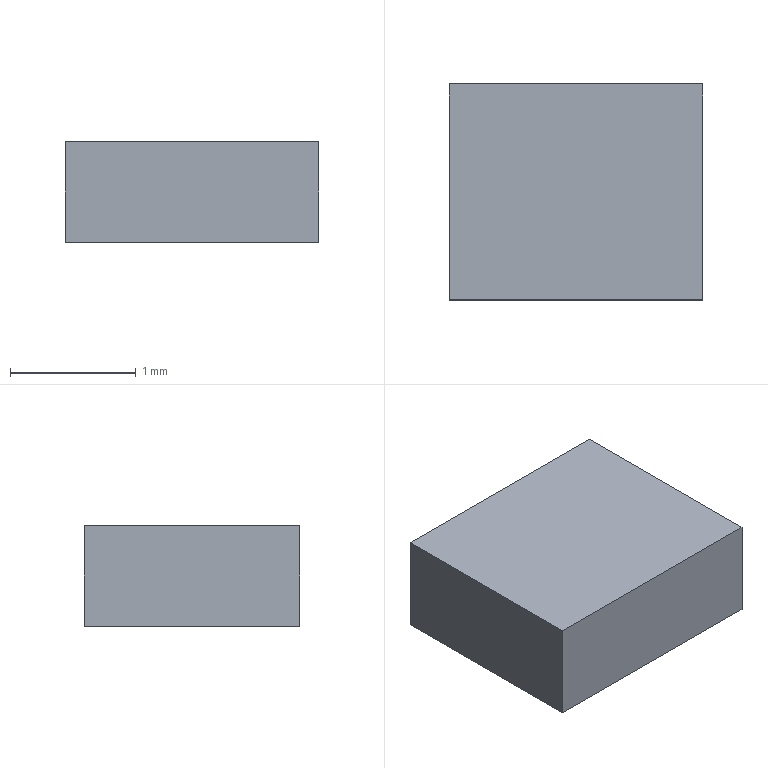Part | Creo | 1 solid | 6 faces | box 2.02 x 1.72 x 0.8 mm | volume 2.78 mm3 | plane 6
STEP:
#1=CARTESIAN_POINT('',(0.,0.,0.));
#2=DIRECTION('',(0.,0.,1.));
#3=DIRECTION('',(1.,0.,0.));
#4=AXIS2_PLACEMENT_3D('',#1,#2,#3);
#5=CARTESIAN_POINT('',(-1.01,-0.86,0.));
#6=VERTEX_POINT('',#5);
#7=CARTESIAN_POINT('',(1.01,-0.86,0.));
#8=VERTEX_POINT('',#7);
#9=CARTESIAN_POINT('',(-1.01,-0.86,0.));
#10=DIRECTION('',(1.,0.,0.));
#11=VECTOR('',#10,2.02);
#12=LINE('',#9,#11);
#13=EDGE_CURVE('',#6,#8,#12,.T.);
#14=ORIENTED_EDGE('',*,*,#13,.T.);
#15=CARTESIAN_POINT('',(1.01,0.86,0.));
#16=VERTEX_POINT('',#15);
#17=CARTESIAN_POINT('',(1.01,-0.86,0.));
#18=DIRECTION('',(0.,1.,0.));
#19=VECTOR('',#18,1.72);
#20=LINE('',#17,#19);
#21=EDGE_CURVE('',#8,#16,#20,.T.);
#22=ORIENTED_EDGE('',*,*,#21,.T.);
#23=CARTESIAN_POINT('',(-1.01,0.86,0.));
#24=VERTEX_POINT('',#23);
#25=CARTESIAN_POINT('',(1.01,0.86,0.));
#26=DIRECTION('',(-1.,0.,0.));
#27=VECTOR('',#26,2.02);
#28=LINE('',#25,#27);
#29=EDGE_CURVE('',#16,#24,#28,.T.);
#30=ORIENTED_EDGE('',*,*,#29,.T.);
#31=CARTESIAN_POINT('',(-1.01,0.86,0.));
#32=DIRECTION('',(0.,-1.,0.));
#33=VECTOR('',#32,1.72);
#34=LINE('',#31,#33);
#35=EDGE_CURVE('',#24,#6,#34,.T.);
#36=ORIENTED_EDGE('',*,*,#35,.T.);
#37=EDGE_LOOP('',(#14,#22,#30,#36));
#38=FACE_OUTER_BOUND('',#37,.F.);
#39=CARTESIAN_POINT('',(0.,0.,0.));
#40=DIRECTION('',(0.,0.,1.));
#41=DIRECTION('',(1.,0.,0.));
#42=AXIS2_PLACEMENT_3D('',#39,#40,#41);
#43=PLANE('',#42);
#44=ADVANCED_FACE('',(#38),#43,.F.);
#45=ORIENTED_EDGE('',*,*,#13,.F.);
#46=CARTESIAN_POINT('',(-1.01,-0.86,0.8));
#47=VERTEX_POINT('',#46);
#48=CARTESIAN_POINT('',(-1.01,-0.86,0.));
#49=DIRECTION('',(0.,0.,1.));
#50=VECTOR('',#49,0.8);
#51=LINE('',#48,#50);
#52=EDGE_CURVE('',#6,#47,#51,.T.);
#53=ORIENTED_EDGE('',*,*,#52,.T.);
#54=CARTESIAN_POINT('',(1.01,-0.86,0.8));
#55=VERTEX_POINT('',#54);
#56=CARTESIAN_POINT('',(-1.01,-0.86,0.8));
#57=DIRECTION('',(1.,0.,0.));
#58=VECTOR('',#57,2.02);
#59=LINE('',#56,#58);
#60=EDGE_CURVE('',#47,#55,#59,.T.);
#61=ORIENTED_EDGE('',*,*,#60,.T.);
#62=CARTESIAN_POINT('',(1.01,-0.86,0.));
#63=DIRECTION('',(0.,0.,1.));
#64=VECTOR('',#63,0.8);
#65=LINE('',#62,#64);
#66=EDGE_CURVE('',#8,#55,#65,.T.);
#67=ORIENTED_EDGE('',*,*,#66,.F.);
#68=EDGE_LOOP('',(#45,#53,#61,#67));
#69=FACE_OUTER_BOUND('',#68,.F.);
#70=CARTESIAN_POINT('',(-1.01,-0.86,0.));
#71=DIRECTION('',(0.,-1.,0.));
#72=DIRECTION('',(1.,0.,0.));
#73=AXIS2_PLACEMENT_3D('',#70,#71,#72);
#74=PLANE('',#73);
#75=ADVANCED_FACE('',(#69),#74,.T.);
#76=ORIENTED_EDGE('',*,*,#35,.F.);
#77=CARTESIAN_POINT('',(-1.01,0.86,0.8));
#78=VERTEX_POINT('',#77);
#79=CARTESIAN_POINT('',(-1.01,0.86,0.));
#80=DIRECTION('',(0.,0.,1.));
#81=VECTOR('',#80,0.8);
#82=LINE('',#79,#81);
#83=EDGE_CURVE('',#24,#78,#82,.T.);
#84=ORIENTED_EDGE('',*,*,#83,.T.);
#85=CARTESIAN_POINT('',(-1.01,0.86,0.8));
#86=DIRECTION('',(0.,-1.,0.));
#87=VECTOR('',#86,1.72);
#88=LINE('',#85,#87);
#89=EDGE_CURVE('',#78,#47,#88,.T.);
#90=ORIENTED_EDGE('',*,*,#89,.T.);
#91=ORIENTED_EDGE('',*,*,#52,.F.);
#92=EDGE_LOOP('',(#76,#84,#90,#91));
#93=FACE_OUTER_BOUND('',#92,.F.);
#94=CARTESIAN_POINT('',(-1.01,0.86,0.));
#95=DIRECTION('',(-1.,0.,0.));
#96=DIRECTION('',(0.,-1.,0.));
#97=AXIS2_PLACEMENT_3D('',#94,#95,#96);
#98=PLANE('',#97);
#99=ADVANCED_FACE('',(#93),#98,.T.);
#100=ORIENTED_EDGE('',*,*,#29,.F.);
#101=CARTESIAN_POINT('',(1.01,0.86,0.8));
#102=VERTEX_POINT('',#101);
#103=CARTESIAN_POINT('',(1.01,0.86,0.));
#104=DIRECTION('',(0.,0.,1.));
#105=VECTOR('',#104,0.8);
#106=LINE('',#103,#105);
#107=EDGE_CURVE('',#16,#102,#106,.T.);
#108=ORIENTED_EDGE('',*,*,#107,.T.);
#109=CARTESIAN_POINT('',(1.01,0.86,0.8));
#110=DIRECTION('',(-1.,0.,0.));
#111=VECTOR('',#110,2.02);
#112=LINE('',#109,#111);
#113=EDGE_CURVE('',#102,#78,#112,.T.);
#114=ORIENTED_EDGE('',*,*,#113,.T.);
#115=ORIENTED_EDGE('',*,*,#83,.F.);
#116=EDGE_LOOP('',(#100,#108,#114,#115));
#117=FACE_OUTER_BOUND('',#116,.F.);
#118=CARTESIAN_POINT('',(1.01,0.86,0.));
#119=DIRECTION('',(0.,1.,0.));
#120=DIRECTION('',(-1.,0.,0.));
#121=AXIS2_PLACEMENT_3D('',#118,#119,#120);
#122=PLANE('',#121);
#123=ADVANCED_FACE('',(#117),#122,.T.);
#124=ORIENTED_EDGE('',*,*,#21,.F.);
#125=ORIENTED_EDGE('',*,*,#66,.T.);
#126=CARTESIAN_POINT('',(1.01,-0.86,0.8));
#127=DIRECTION('',(0.,1.,0.));
#128=VECTOR('',#127,1.72);
#129=LINE('',#126,#128);
#130=EDGE_CURVE('',#55,#102,#129,.T.);
#131=ORIENTED_EDGE('',*,*,#130,.T.);
#132=ORIENTED_EDGE('',*,*,#107,.F.);
#133=EDGE_LOOP('',(#124,#125,#131,#132));
#134=FACE_OUTER_BOUND('',#133,.F.);
#135=CARTESIAN_POINT('',(1.01,-0.86,0.));
#136=DIRECTION('',(1.,0.,0.));
#137=DIRECTION('',(0.,1.,0.));
#138=AXIS2_PLACEMENT_3D('',#135,#136,#137);
#139=PLANE('',#138);
#140=ADVANCED_FACE('',(#134),#139,.T.);
#141=ORIENTED_EDGE('',*,*,#60,.F.);
#142=ORIENTED_EDGE('',*,*,#89,.F.);
#143=ORIENTED_EDGE('',*,*,#113,.F.);
#144=ORIENTED_EDGE('',*,*,#130,.F.);
#145=EDGE_LOOP('',(#141,#142,#143,#144));
#146=FACE_OUTER_BOUND('',#145,.F.);
#147=CARTESIAN_POINT('',(0.,0.,0.8));
#148=DIRECTION('',(0.,0.,1.));
#149=DIRECTION('',(1.,0.,0.));
#150=AXIS2_PLACEMENT_3D('',#147,#148,#149);
#151=PLANE('',#150);
#152=ADVANCED_FACE('',(#146),#151,.T.);
#153=CLOSED_SHELL('',(#44,#75,#99,#123,#140,#152));
#154=MANIFOLD_SOLID_BREP('',#153);
#155=(LENGTH_UNIT()NAMED_UNIT(*)SI_UNIT(.MILLI.,.METRE.));
#156=UNCERTAINTY_MEASURE_WITH_UNIT(LENGTH_MEASURE(0.0002771),#155,'','');
#157=(NAMED_UNIT(*)PLANE_ANGLE_UNIT()SI_UNIT($,.RADIAN.));
#158=PLANE_ANGLE_MEASURE_WITH_UNIT(PLANE_ANGLE_MEASURE(0.01745),#157);
#159=(CONVERSION_BASED_UNIT('DEGREE',#158)NAMED_UNIT(*)PLANE_ANGLE_UNIT());
#160=(NAMED_UNIT(*)SI_UNIT($,.STERADIAN.)SOLID_ANGLE_UNIT());
#161=(GEOMETRIC_REPRESENTATION_CONTEXT(3)GLOBAL_UNCERTAINTY_ASSIGNED_CONTEXT((#156))GLOBAL_UNIT_ASSIGNED_CONTEXT((#155,#159,#160))REPRESENTATION_CONTEXT('',''));
#162=ADVANCED_BREP_SHAPE_REPRESENTATION('',(#4,#154),#161);